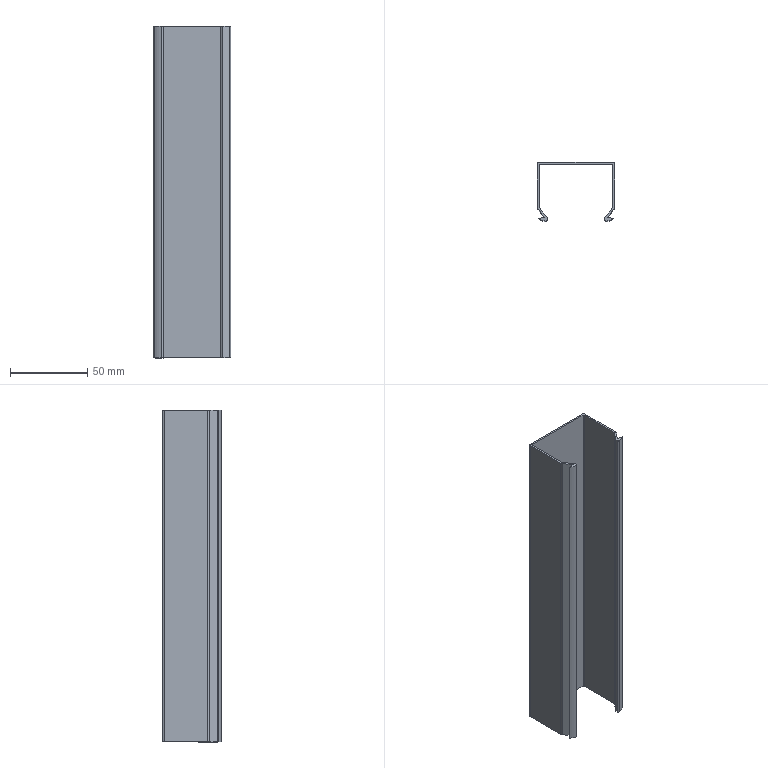Part | STEP file | 31E-01000CC12 | 1 solid | 28 faces | box 50 x 38.192 x 215 mm | volume 35398 mm3 | plane 16 | cylinder 12 | commonest cylinder face diameters 1 x4 2 x4 4 x2 26 x2
STEP:
#1=CARTESIAN_POINT('',(27.993,8.298,215.));
#2=VERTEX_POINT('',#1);
#3=CARTESIAN_POINT('',(32.281,3.187,215.));
#4=VERTEX_POINT('',#3);
#5=CARTESIAN_POINT('',(30.137,5.743,215.));
#6=DIRECTION('',(0.6428,-0.766,0.));
#7=VECTOR('',#6,1.);
#8=LINE('',#5,#7);
#9=EDGE_CURVE('',#2,#4,#8,.T.);
#10=ORIENTED_EDGE('',*,*,#9,.F.);
#11=CARTESIAN_POINT('',(27.993,8.298,0.));
#12=VERTEX_POINT('',#11);
#13=CARTESIAN_POINT('',(27.993,8.298,107.5));
#14=DIRECTION('',(0.,0.,-1.));
#15=VECTOR('',#14,1.);
#16=LINE('',#13,#15);
#17=EDGE_CURVE('',#2,#12,#16,.T.);
#18=ORIENTED_EDGE('',*,*,#17,.T.);
#19=CARTESIAN_POINT('',(32.281,3.187,0.));
#20=VERTEX_POINT('',#19);
#21=CARTESIAN_POINT('',(30.137,5.743,0.));
#22=DIRECTION('',(0.6428,-0.766,0.));
#23=VECTOR('',#22,1.);
#24=LINE('',#21,#23);
#25=EDGE_CURVE('',#12,#20,#24,.T.);
#26=ORIENTED_EDGE('',*,*,#25,.T.);
#27=CARTESIAN_POINT('',(32.281,3.187,107.5));
#28=DIRECTION('',(0.,0.,-1.));
#29=VECTOR('',#28,1.);
#30=LINE('',#27,#29);
#31=EDGE_CURVE('',#4,#20,#30,.T.);
#32=ORIENTED_EDGE('',*,*,#31,.F.);
#33=EDGE_LOOP('',(#10,#18,#26,#32));
#34=FACE_OUTER_BOUND('',#33,.T.);
#35=CARTESIAN_POINT('',(27.525,8.856,215.));
#36=DIRECTION('',(0.766,0.6428,0.));
#37=DIRECTION('',(-0.6428,0.766,0.));
#38=AXIS2_PLACEMENT_3D('',#35,#36,#37);
#39=PLANE('',#38);
#40=ADVANCED_FACE('',(#34),#39,.F.);
#41=CARTESIAN_POINT('',(76.325,9.293,215.));
#42=VERTEX_POINT('',#41);
#43=CARTESIAN_POINT('',(71.299,3.304,215.));
#44=VERTEX_POINT('',#43);
#45=CARTESIAN_POINT('',(73.812,6.298,215.));
#46=DIRECTION('',(-0.6428,-0.766,0.));
#47=VECTOR('',#46,1.);
#48=LINE('',#45,#47);
#49=EDGE_CURVE('',#42,#44,#48,.T.);
#50=ORIENTED_EDGE('',*,*,#49,.T.);
#51=CARTESIAN_POINT('',(71.182,2.983,215.));
#52=VERTEX_POINT('',#51);
#53=CARTESIAN_POINT('',(71.682,2.983,215.));
#54=DIRECTION('',(0.,0.,1.));
#55=AXIS2_PLACEMENT_3D('',#53,#54,$);
#56=CIRCLE('',#55,0.5);
#57=EDGE_CURVE('',#44,#52,#56,.T.);
#58=ORIENTED_EDGE('',*,*,#57,.T.);
#59=CARTESIAN_POINT('',(71.182,1.665,215.));
#60=VERTEX_POINT('',#59);
#61=CARTESIAN_POINT('',(71.182,2.324,215.));
#62=DIRECTION('',(0.,-1.,0.));
#63=VECTOR('',#62,1.);
#64=LINE('',#61,#63);
#65=EDGE_CURVE('',#52,#60,#64,.T.);
#66=ORIENTED_EDGE('',*,*,#65,.T.);
#67=CARTESIAN_POINT('',(72.397,0.6877,215.));
#68=VERTEX_POINT('',#67);
#69=CARTESIAN_POINT('',(72.182,1.665,215.));
#70=DIRECTION('',(0.,0.,1.));
#71=AXIS2_PLACEMENT_3D('',#69,#70,$);
#72=CIRCLE('',#71,1.);
#73=EDGE_CURVE('',#60,#68,#72,.T.);
#74=ORIENTED_EDGE('',*,*,#73,.T.);
#75=CARTESIAN_POINT('',(76.707,2.493,215.));
#76=VERTEX_POINT('',#75);
#77=CARTESIAN_POINT('',(69.613,13.386,215.));
#78=DIRECTION('',(0.,0.,1.));
#79=AXIS2_PLACEMENT_3D('',#77,#78,$);
#80=CIRCLE('',#79,13.);
#81=EDGE_CURVE('',#68,#76,#80,.T.);
#82=ORIENTED_EDGE('',*,*,#81,.T.);
#83=CARTESIAN_POINT('',(72.768,3.187,215.));
#84=VERTEX_POINT('',#83);
#85=CARTESIAN_POINT('',(74.738,2.84,215.));
#86=DIRECTION('',(-0.9848,0.1736,0.));
#87=VECTOR('',#86,1.);
#88=LINE('',#85,#87);
#89=EDGE_CURVE('',#76,#84,#88,.T.);
#90=ORIENTED_EDGE('',*,*,#89,.T.);
#91=CARTESIAN_POINT('',(77.057,8.298,215.));
#92=VERTEX_POINT('',#91);
#93=CARTESIAN_POINT('',(74.912,5.743,215.));
#94=DIRECTION('',(0.6428,0.766,0.));
#95=VECTOR('',#94,1.);
#96=LINE('',#93,#95);
#97=EDGE_CURVE('',#84,#92,#96,.T.);
#98=ORIENTED_EDGE('',*,*,#97,.T.);
#99=CARTESIAN_POINT('',(77.525,9.584,215.));
#100=VERTEX_POINT('',#99);
#101=CARTESIAN_POINT('',(75.525,9.584,215.));
#102=DIRECTION('',(0.,0.,1.));
#103=AXIS2_PLACEMENT_3D('',#101,#102,$);
#104=CIRCLE('',#103,2.);
#105=EDGE_CURVE('',#92,#100,#104,.T.);
#106=ORIENTED_EDGE('',*,*,#105,.T.);
#107=CARTESIAN_POINT('',(77.525,37.856,215.));
#108=VERTEX_POINT('',#107);
#109=CARTESIAN_POINT('',(77.525,23.72,215.));
#110=DIRECTION('',(0.,1.,0.));
#111=VECTOR('',#110,1.);
#112=LINE('',#109,#111);
#113=EDGE_CURVE('',#100,#108,#112,.T.);
#114=ORIENTED_EDGE('',*,*,#113,.T.);
#115=CARTESIAN_POINT('',(76.525,38.856,215.));
#116=VERTEX_POINT('',#115);
#117=CARTESIAN_POINT('',(76.525,37.856,215.));
#118=DIRECTION('',(0.,0.,1.));
#119=AXIS2_PLACEMENT_3D('',#117,#118,$);
#120=CIRCLE('',#119,1.);
#121=EDGE_CURVE('',#108,#116,#120,.T.);
#122=ORIENTED_EDGE('',*,*,#121,.T.);
#123=CARTESIAN_POINT('',(28.525,38.856,215.));
#124=VERTEX_POINT('',#123);
#125=CARTESIAN_POINT('',(52.525,38.856,215.));
#126=DIRECTION('',(-1.,0.,0.));
#127=VECTOR('',#126,1.);
#128=LINE('',#125,#127);
#129=EDGE_CURVE('',#116,#124,#128,.T.);
#130=ORIENTED_EDGE('',*,*,#129,.T.);
#131=CARTESIAN_POINT('',(27.525,37.856,215.));
#132=VERTEX_POINT('',#131);
#133=CARTESIAN_POINT('',(28.525,37.856,215.));
#134=DIRECTION('',(0.,0.,1.));
#135=AXIS2_PLACEMENT_3D('',#133,#134,$);
#136=CIRCLE('',#135,1.);
#137=EDGE_CURVE('',#124,#132,#136,.T.);
#138=ORIENTED_EDGE('',*,*,#137,.T.);
#139=CARTESIAN_POINT('',(27.525,9.584,215.));
#140=VERTEX_POINT('',#139);
#141=CARTESIAN_POINT('',(27.525,23.72,215.));
#142=DIRECTION('',(0.,-1.,0.));
#143=VECTOR('',#142,1.);
#144=LINE('',#141,#143);
#145=EDGE_CURVE('',#132,#140,#144,.T.);
#146=ORIENTED_EDGE('',*,*,#145,.T.);
#147=CARTESIAN_POINT('',(29.525,9.584,215.));
#148=DIRECTION('',(0.,0.,1.));
#149=AXIS2_PLACEMENT_3D('',#147,#148,$);
#150=CIRCLE('',#149,2.);
#151=EDGE_CURVE('',#140,#2,#150,.T.);
#152=ORIENTED_EDGE('',*,*,#151,.T.);
#153=ORIENTED_EDGE('',*,*,#9,.T.);
#154=CARTESIAN_POINT('',(28.342,2.493,215.));
#155=VERTEX_POINT('',#154);
#156=CARTESIAN_POINT('',(30.312,2.84,215.));
#157=DIRECTION('',(-0.9848,-0.1736,0.));
#158=VECTOR('',#157,1.);
#159=LINE('',#156,#158);
#160=EDGE_CURVE('',#4,#155,#159,.T.);
#161=ORIENTED_EDGE('',*,*,#160,.T.);
#162=CARTESIAN_POINT('',(32.653,0.6877,215.));
#163=VERTEX_POINT('',#162);
#164=CARTESIAN_POINT('',(35.437,13.386,215.));
#165=DIRECTION('',(0.,0.,1.));
#166=AXIS2_PLACEMENT_3D('',#164,#165,$);
#167=CIRCLE('',#166,13.);
#168=EDGE_CURVE('',#155,#163,#167,.T.);
#169=ORIENTED_EDGE('',*,*,#168,.T.);
#170=CARTESIAN_POINT('',(33.867,1.665,215.));
#171=VERTEX_POINT('',#170);
#172=CARTESIAN_POINT('',(32.867,1.665,215.));
#173=DIRECTION('',(0.,0.,1.));
#174=AXIS2_PLACEMENT_3D('',#172,#173,$);
#175=CIRCLE('',#174,1.);
#176=EDGE_CURVE('',#163,#171,#175,.T.);
#177=ORIENTED_EDGE('',*,*,#176,.T.);
#178=CARTESIAN_POINT('',(33.867,2.983,215.));
#179=VERTEX_POINT('',#178);
#180=CARTESIAN_POINT('',(33.867,2.324,215.));
#181=DIRECTION('',(0.,1.,0.));
#182=VECTOR('',#181,1.);
#183=LINE('',#180,#182);
#184=EDGE_CURVE('',#171,#179,#183,.T.);
#185=ORIENTED_EDGE('',*,*,#184,.T.);
#186=CARTESIAN_POINT('',(33.75,3.304,215.));
#187=VERTEX_POINT('',#186);
#188=CARTESIAN_POINT('',(33.367,2.983,215.));
#189=DIRECTION('',(0.,0.,1.));
#190=AXIS2_PLACEMENT_3D('',#188,#189,$);
#191=CIRCLE('',#190,0.5);
#192=EDGE_CURVE('',#179,#187,#191,.T.);
#193=ORIENTED_EDGE('',*,*,#192,.T.);
#194=CARTESIAN_POINT('',(28.725,9.293,215.));
#195=VERTEX_POINT('',#194);
#196=CARTESIAN_POINT('',(31.237,6.298,215.));
#197=DIRECTION('',(-0.6428,0.766,0.));
#198=VECTOR('',#197,1.);
#199=LINE('',#196,#198);
#200=EDGE_CURVE('',#187,#195,#199,.T.);
#201=ORIENTED_EDGE('',*,*,#200,.T.);
#202=CARTESIAN_POINT('',(28.725,37.156,215.));
#203=VERTEX_POINT('',#202);
#204=CARTESIAN_POINT('',(28.725,23.225,215.));
#205=DIRECTION('',(0.,1.,0.));
#206=VECTOR('',#205,1.);
#207=LINE('',#204,#206);
#208=EDGE_CURVE('',#195,#203,#207,.T.);
#209=ORIENTED_EDGE('',*,*,#208,.T.);
#210=CARTESIAN_POINT('',(29.225,37.656,215.));
#211=VERTEX_POINT('',#210);
#212=CARTESIAN_POINT('',(28.725,37.156,215.));
#213=CARTESIAN_POINT('',(28.725,37.219,215.));
#214=CARTESIAN_POINT('',(28.735,37.282,215.));
#215=CARTESIAN_POINT('',(28.754,37.343,215.));
#216=CARTESIAN_POINT('',(28.812,37.456,215.));
#217=CARTESIAN_POINT('',(28.902,37.546,215.));
#218=CARTESIAN_POINT('',(28.954,37.583,215.));
#219=CARTESIAN_POINT('',(29.039,37.627,215.));
#220=CARTESIAN_POINT('',(29.131,37.649,215.));
#221=CARTESIAN_POINT('',(29.162,37.654,215.));
#222=CARTESIAN_POINT('',(29.193,37.656,215.));
#223=CARTESIAN_POINT('',(29.225,37.656,215.));
#224=B_SPLINE_CURVE_WITH_KNOTS('',5,(#212,#213,#214,#215,#216,#217,#218,#219,#220,#221,#222,#223),.UNSPECIFIED.,.F.,.U.,(6,3,3,6),(0.,0.4443,0.8886,1.11),.UNSPECIFIED.);
#225=EDGE_CURVE('',#203,#211,#224,.T.);
#226=ORIENTED_EDGE('',*,*,#225,.T.);
#227=CARTESIAN_POINT('',(75.825,37.656,215.));
#228=VERTEX_POINT('',#227);
#229=CARTESIAN_POINT('',(52.525,37.656,215.));
#230=DIRECTION('',(1.,0.,0.));
#231=VECTOR('',#230,1.);
#232=LINE('',#229,#231);
#233=EDGE_CURVE('',#211,#228,#232,.T.);
#234=ORIENTED_EDGE('',*,*,#233,.T.);
#235=CARTESIAN_POINT('',(76.325,37.156,215.));
#236=VERTEX_POINT('',#235);
#237=CARTESIAN_POINT('',(75.825,37.656,215.));
#238=CARTESIAN_POINT('',(75.888,37.656,215.));
#239=CARTESIAN_POINT('',(75.95,37.646,215.));
#240=CARTESIAN_POINT('',(76.011,37.627,215.));
#241=CARTESIAN_POINT('',(76.124,37.569,215.));
#242=CARTESIAN_POINT('',(76.214,37.479,215.));
#243=CARTESIAN_POINT('',(76.252,37.427,215.));
#244=CARTESIAN_POINT('',(76.295,37.342,215.));
#245=CARTESIAN_POINT('',(76.317,37.25,215.));
#246=CARTESIAN_POINT('',(76.322,37.219,215.));
#247=CARTESIAN_POINT('',(76.325,37.187,215.));
#248=CARTESIAN_POINT('',(76.325,37.156,215.));
#249=B_SPLINE_CURVE_WITH_KNOTS('',5,(#237,#238,#239,#240,#241,#242,#243,#244,#245,#246,#247,#248),.UNSPECIFIED.,.F.,.U.,(6,3,3,6),(0.,0.4443,0.8886,1.11),.UNSPECIFIED.);
#250=EDGE_CURVE('',#228,#236,#249,.T.);
#251=ORIENTED_EDGE('',*,*,#250,.T.);
#252=CARTESIAN_POINT('',(76.325,23.225,215.));
#253=DIRECTION('',(0.,-1.,0.));
#254=VECTOR('',#253,1.);
#255=LINE('',#252,#254);
#256=EDGE_CURVE('',#236,#42,#255,.T.);
#257=ORIENTED_EDGE('',*,*,#256,.T.);
#258=EDGE_LOOP('',(#50,#58,#66,#74,#82,#90,#98,#106,#114,#122,#130,#138,#146,#152,#153,#161,#169,#177,#185,#193,#201,#209,#226,#234,#251,#257));
#259=FACE_OUTER_BOUND('',#258,.T.);
#260=CARTESIAN_POINT('',(35.437,13.386,215.));
#261=DIRECTION('',(0.,0.,1.));
#262=DIRECTION('',(1.,0.,0.));
#263=AXIS2_PLACEMENT_3D('',#260,#261,#262);
#264=PLANE('',#263);
#265=ADVANCED_FACE('',(#259),#264,.T.);
#266=ORIENTED_EDGE('',*,*,#151,.F.);
#267=CARTESIAN_POINT('',(27.525,9.584,0.));
#268=VERTEX_POINT('',#267);
#269=CARTESIAN_POINT('',(27.525,9.584,215.));
#270=DIRECTION('',(0.,0.,-1.));
#271=VECTOR('',#270,1.);
#272=LINE('',#269,#271);
#273=EDGE_CURVE('',#268,#140,#272,.F.);
#274=ORIENTED_EDGE('',*,*,#273,.F.);
#275=CARTESIAN_POINT('',(29.525,9.584,0.));
#276=DIRECTION('',(0.,0.,-1.));
#277=AXIS2_PLACEMENT_3D('',#275,#276,$);
#278=CIRCLE('',#277,2.);
#279=EDGE_CURVE('',#12,#268,#278,.T.);
#280=ORIENTED_EDGE('',*,*,#279,.F.);
#281=ORIENTED_EDGE('',*,*,#17,.F.);
#282=EDGE_LOOP('',(#266,#274,#280,#281));
#283=FACE_OUTER_BOUND('',#282,.T.);
#284=CARTESIAN_POINT('',(29.525,9.584,215.));
#285=DIRECTION('',(0.,0.,-1.));
#286=DIRECTION('',(1.,0.,0.));
#287=AXIS2_PLACEMENT_3D('',#284,#285,#286);
#288=CYLINDRICAL_SURFACE('',#287,2.);
#289=ADVANCED_FACE('',(#283),#288,.T.);
#290=CARTESIAN_POINT('',(71.182,2.983,0.));
#291=VERTEX_POINT('',#290);
#292=CARTESIAN_POINT('',(71.182,1.665,0.));
#293=VERTEX_POINT('',#292);
#294=CARTESIAN_POINT('',(71.182,2.324,0.));
#295=DIRECTION('',(0.,-1.,0.));
#296=VECTOR('',#295,1.);
#297=LINE('',#294,#296);
#298=EDGE_CURVE('',#291,#293,#297,.T.);
#299=ORIENTED_EDGE('',*,*,#298,.F.);
#300=CARTESIAN_POINT('',(71.299,3.304,0.));
#301=VERTEX_POINT('',#300);
#302=CARTESIAN_POINT('',(71.182,2.983,0.));
#303=CARTESIAN_POINT('',(71.182,3.038,0.));
#304=CARTESIAN_POINT('',(71.19,3.094,0.));
#305=CARTESIAN_POINT('',(71.206,3.149,0.));
#306=CARTESIAN_POINT('',(71.235,3.213,0.));
#307=CARTESIAN_POINT('',(71.274,3.271,0.));
#308=CARTESIAN_POINT('',(71.282,3.282,0.));
#309=CARTESIAN_POINT('',(71.29,3.293,0.));
#310=CARTESIAN_POINT('',(71.299,3.304,0.));
#311=B_SPLINE_CURVE_WITH_KNOTS('',5,(#302,#303,#304,#305,#306,#307,#308,#309,#310),.UNSPECIFIED.,.F.,.U.,(6,3,6),(0.,0.3949,0.4936),.UNSPECIFIED.);
#312=EDGE_CURVE('',#291,#301,#311,.T.);
#313=ORIENTED_EDGE('',*,*,#312,.T.);
#314=CARTESIAN_POINT('',(76.325,9.293,0.));
#315=VERTEX_POINT('',#314);
#316=CARTESIAN_POINT('',(73.812,6.298,0.));
#317=DIRECTION('',(-0.6428,-0.766,0.));
#318=VECTOR('',#317,1.);
#319=LINE('',#316,#318);
#320=EDGE_CURVE('',#315,#301,#319,.T.);
#321=ORIENTED_EDGE('',*,*,#320,.F.);
#322=CARTESIAN_POINT('',(76.325,37.156,0.));
#323=VERTEX_POINT('',#322);
#324=CARTESIAN_POINT('',(76.325,23.225,0.));
#325=DIRECTION('',(0.,-1.,0.));
#326=VECTOR('',#325,1.);
#327=LINE('',#324,#326);
#328=EDGE_CURVE('',#323,#315,#327,.T.);
#329=ORIENTED_EDGE('',*,*,#328,.F.);
#330=CARTESIAN_POINT('',(75.825,37.656,0.));
#331=VERTEX_POINT('',#330);
#332=CARTESIAN_POINT('',(75.825,37.156,0.));
#333=DIRECTION('',(0.,0.,1.));
#334=AXIS2_PLACEMENT_3D('',#332,#333,$);
#335=CIRCLE('',#334,0.5);
#336=EDGE_CURVE('',#323,#331,#335,.T.);
#337=ORIENTED_EDGE('',*,*,#336,.T.);
#338=CARTESIAN_POINT('',(29.225,37.656,0.));
#339=VERTEX_POINT('',#338);
#340=CARTESIAN_POINT('',(52.525,37.656,0.));
#341=DIRECTION('',(1.,0.,0.));
#342=VECTOR('',#341,1.);
#343=LINE('',#340,#342);
#344=EDGE_CURVE('',#339,#331,#343,.T.);
#345=ORIENTED_EDGE('',*,*,#344,.F.);
#346=CARTESIAN_POINT('',(28.725,37.156,0.));
#347=VERTEX_POINT('',#346);
#348=CARTESIAN_POINT('',(29.225,37.156,0.));
#349=DIRECTION('',(0.,0.,1.));
#350=AXIS2_PLACEMENT_3D('',#348,#349,$);
#351=CIRCLE('',#350,0.5);
#352=EDGE_CURVE('',#339,#347,#351,.T.);
#353=ORIENTED_EDGE('',*,*,#352,.T.);
#354=CARTESIAN_POINT('',(28.725,9.293,0.));
#355=VERTEX_POINT('',#354);
#356=CARTESIAN_POINT('',(28.725,23.225,0.));
#357=DIRECTION('',(0.,1.,0.));
#358=VECTOR('',#357,1.);
#359=LINE('',#356,#358);
#360=EDGE_CURVE('',#355,#347,#359,.T.);
#361=ORIENTED_EDGE('',*,*,#360,.F.);
#362=CARTESIAN_POINT('',(33.75,3.304,0.));
#363=VERTEX_POINT('',#362);
#364=CARTESIAN_POINT('',(31.237,6.298,0.));
#365=DIRECTION('',(-0.6428,0.766,0.));
#366=VECTOR('',#365,1.);
#367=LINE('',#364,#366);
#368=EDGE_CURVE('',#363,#355,#367,.T.);
#369=ORIENTED_EDGE('',*,*,#368,.F.);
#370=CARTESIAN_POINT('',(33.867,2.983,0.));
#371=VERTEX_POINT('',#370);
#372=CARTESIAN_POINT('',(33.75,3.304,0.));
#373=CARTESIAN_POINT('',(33.786,3.261,0.));
#374=CARTESIAN_POINT('',(33.816,3.213,0.));
#375=CARTESIAN_POINT('',(33.839,3.162,0.));
#376=CARTESIAN_POINT('',(33.858,3.094,0.));
#377=CARTESIAN_POINT('',(33.866,3.024,0.));
#378=CARTESIAN_POINT('',(33.867,3.01,0.));
#379=CARTESIAN_POINT('',(33.867,2.997,0.));
#380=CARTESIAN_POINT('',(33.867,2.983,0.));
#381=B_SPLINE_CURVE_WITH_KNOTS('',5,(#372,#373,#374,#375,#376,#377,#378,#379,#380),.UNSPECIFIED.,.F.,.U.,(6,3,6),(0.,0.3949,0.4936),.UNSPECIFIED.);
#382=EDGE_CURVE('',#363,#371,#381,.T.);
#383=ORIENTED_EDGE('',*,*,#382,.T.);
#384=CARTESIAN_POINT('',(33.867,1.665,0.));
#385=VERTEX_POINT('',#384);
#386=CARTESIAN_POINT('',(33.867,2.324,0.));
#387=DIRECTION('',(0.,1.,0.));
#388=VECTOR('',#387,1.);
#389=LINE('',#386,#388);
#390=EDGE_CURVE('',#385,#371,#389,.T.);
#391=ORIENTED_EDGE('',*,*,#390,.F.);
#392=CARTESIAN_POINT('',(32.653,0.6877,0.));
#393=VERTEX_POINT('',#392);
#394=CARTESIAN_POINT('',(32.867,1.665,0.));
#395=DIRECTION('',(0.,0.,1.));
#396=AXIS2_PLACEMENT_3D('',#394,#395,$);
#397=CIRCLE('',#396,1.);
#398=EDGE_CURVE('',#393,#385,#397,.T.);
#399=ORIENTED_EDGE('',*,*,#398,.F.);
#400=CARTESIAN_POINT('',(28.342,2.493,0.));
#401=VERTEX_POINT('',#400);
#402=CARTESIAN_POINT('',(35.437,13.386,0.));
#403=DIRECTION('',(0.,0.,1.));
#404=AXIS2_PLACEMENT_3D('',#402,#403,$);
#405=CIRCLE('',#404,13.);
#406=EDGE_CURVE('',#401,#393,#405,.T.);
#407=ORIENTED_EDGE('',*,*,#406,.F.);
#408=CARTESIAN_POINT('',(30.312,2.84,0.));
#409=DIRECTION('',(-0.9848,-0.1736,0.));
#410=VECTOR('',#409,1.);
#411=LINE('',#408,#410);
#412=EDGE_CURVE('',#20,#401,#411,.T.);
#413=ORIENTED_EDGE('',*,*,#412,.F.);
#414=ORIENTED_EDGE('',*,*,#25,.F.);
#415=ORIENTED_EDGE('',*,*,#279,.T.);
#416=CARTESIAN_POINT('',(27.525,37.856,0.));
#417=VERTEX_POINT('',#416);
#418=CARTESIAN_POINT('',(27.525,23.72,0.));
#419=DIRECTION('',(0.,-1.,0.));
#420=VECTOR('',#419,1.);
#421=LINE('',#418,#420);
#422=EDGE_CURVE('',#417,#268,#421,.T.);
#423=ORIENTED_EDGE('',*,*,#422,.F.);
#424=CARTESIAN_POINT('',(28.525,38.856,0.));
#425=VERTEX_POINT('',#424);
#426=CARTESIAN_POINT('',(27.525,37.856,0.));
#427=CARTESIAN_POINT('',(27.525,37.954,0.));
#428=CARTESIAN_POINT('',(27.537,38.052,0.));
#429=CARTESIAN_POINT('',(27.561,38.148,0.));
#430=CARTESIAN_POINT('',(27.632,38.332,0.));
#431=CARTESIAN_POINT('',(27.745,38.494,0.));
#432=CARTESIAN_POINT('',(27.812,38.567,0.));
#433=CARTESIAN_POINT('',(27.961,38.696,0.));
#434=CARTESIAN_POINT('',(28.137,38.786,0.));
#435=CARTESIAN_POINT('',(28.23,38.819,0.));
#436=CARTESIAN_POINT('',(28.346,38.846,0.));
#437=CARTESIAN_POINT('',(28.464,38.855,0.));
#438=CARTESIAN_POINT('',(28.484,38.856,0.));
#439=CARTESIAN_POINT('',(28.505,38.856,0.));
#440=CARTESIAN_POINT('',(28.525,38.856,0.));
#441=B_SPLINE_CURVE_WITH_KNOTS('',5,(#426,#427,#428,#429,#430,#431,#432,#433,#434,#435,#436,#437,#438,#439,#440),.UNSPECIFIED.,.F.,.U.,(6,3,3,3,6),(0.,0.6928,1.386,2.078,2.221),.UNSPECIFIED.);
#442=EDGE_CURVE('',#417,#425,#441,.T.);
#443=ORIENTED_EDGE('',*,*,#442,.T.);
#444=CARTESIAN_POINT('',(76.525,38.856,0.));
#445=VERTEX_POINT('',#444);
#446=CARTESIAN_POINT('',(52.525,38.856,0.));
#447=DIRECTION('',(-1.,0.,0.));
#448=VECTOR('',#447,1.);
#449=LINE('',#446,#448);
#450=EDGE_CURVE('',#445,#425,#449,.T.);
#451=ORIENTED_EDGE('',*,*,#450,.F.);
#452=CARTESIAN_POINT('',(77.525,37.856,0.));
#453=VERTEX_POINT('',#452);
#454=CARTESIAN_POINT('',(76.525,38.856,0.));
#455=CARTESIAN_POINT('',(76.623,38.856,0.));
#456=CARTESIAN_POINT('',(76.721,38.844,0.));
#457=CARTESIAN_POINT('',(76.817,38.82,0.));
#458=CARTESIAN_POINT('',(77.001,38.749,0.));
#459=CARTESIAN_POINT('',(77.163,38.636,0.));
#460=CARTESIAN_POINT('',(77.236,38.569,0.));
#461=CARTESIAN_POINT('',(77.365,38.42,0.));
#462=CARTESIAN_POINT('',(77.454,38.244,0.));
#463=CARTESIAN_POINT('',(77.488,38.151,0.));
#464=CARTESIAN_POINT('',(77.514,38.035,0.));
#465=CARTESIAN_POINT('',(77.523,37.917,0.));
#466=CARTESIAN_POINT('',(77.524,37.897,0.));
#467=CARTESIAN_POINT('',(77.525,37.876,0.));
#468=CARTESIAN_POINT('',(77.525,37.856,0.));
#469=B_SPLINE_CURVE_WITH_KNOTS('',5,(#454,#455,#456,#457,#458,#459,#460,#461,#462,#463,#464,#465,#466,#467,#468),.UNSPECIFIED.,.F.,.U.,(6,3,3,3,6),(0.,0.6928,1.386,2.078,2.221),.UNSPECIFIED.);
#470=EDGE_CURVE('',#445,#453,#469,.T.);
#471=ORIENTED_EDGE('',*,*,#470,.T.);
#472=CARTESIAN_POINT('',(77.525,9.584,0.));
#473=VERTEX_POINT('',#472);
#474=CARTESIAN_POINT('',(77.525,23.72,0.));
#475=DIRECTION('',(0.,1.,0.));
#476=VECTOR('',#475,1.);
#477=LINE('',#474,#476);
#478=EDGE_CURVE('',#473,#453,#477,.T.);
#479=ORIENTED_EDGE('',*,*,#478,.F.);
#480=CARTESIAN_POINT('',(77.057,8.298,0.));
#481=VERTEX_POINT('',#480);
#482=CARTESIAN_POINT('',(77.525,9.584,0.));
#483=CARTESIAN_POINT('',(77.525,9.361,0.));
#484=CARTESIAN_POINT('',(77.494,9.137,0.));
#485=CARTESIAN_POINT('',(77.431,8.92,0.));
#486=CARTESIAN_POINT('',(77.316,8.662,0.));
#487=CARTESIAN_POINT('',(77.16,8.431,0.));
#488=CARTESIAN_POINT('',(77.127,8.385,0.));
#489=CARTESIAN_POINT('',(77.093,8.341,0.));
#490=CARTESIAN_POINT('',(77.057,8.298,0.));
#491=B_SPLINE_CURVE_WITH_KNOTS('',5,(#482,#483,#484,#485,#486,#487,#488,#489,#490),.UNSPECIFIED.,.F.,.U.,(6,3,6),(0.,1.58,1.974),.UNSPECIFIED.);
#492=EDGE_CURVE('',#473,#481,#491,.T.);
#493=ORIENTED_EDGE('',*,*,#492,.T.);
#494=CARTESIAN_POINT('',(72.768,3.187,0.));
#495=VERTEX_POINT('',#494);
#496=CARTESIAN_POINT('',(74.912,5.743,0.));
#497=DIRECTION('',(0.6428,0.766,0.));
#498=VECTOR('',#497,1.);
#499=LINE('',#496,#498);
#500=EDGE_CURVE('',#495,#481,#499,.T.);
#501=ORIENTED_EDGE('',*,*,#500,.F.);
#502=CARTESIAN_POINT('',(76.707,2.493,0.));
#503=VERTEX_POINT('',#502);
#504=CARTESIAN_POINT('',(74.738,2.84,0.));
#505=DIRECTION('',(-0.9848,0.1736,0.));
#506=VECTOR('',#505,1.);
#507=LINE('',#504,#506);
#508=EDGE_CURVE('',#503,#495,#507,.T.);
#509=ORIENTED_EDGE('',*,*,#508,.F.);
#510=CARTESIAN_POINT('',(72.397,0.6877,0.));
#511=VERTEX_POINT('',#510);
#512=CARTESIAN_POINT('',(69.613,13.386,0.));
#513=DIRECTION('',(0.,0.,1.));
#514=AXIS2_PLACEMENT_3D('',#512,#513,$);
#515=CIRCLE('',#514,13.);
#516=EDGE_CURVE('',#511,#503,#515,.T.);
#517=ORIENTED_EDGE('',*,*,#516,.F.);
#518=CARTESIAN_POINT('',(72.182,1.665,0.));
#519=DIRECTION('',(0.,0.,1.));
#520=AXIS2_PLACEMENT_3D('',#518,#519,$);
#521=CIRCLE('',#520,1.);
#522=EDGE_CURVE('',#293,#511,#521,.T.);
#523=ORIENTED_EDGE('',*,*,#522,.F.);
#524=EDGE_LOOP('',(#299,#313,#321,#329,#337,#345,#353,#361,#369,#383,#391,#399,#407,#413,#414,#415,#423,#443,#451,#471,#479,#493,#501,#509,#517,#523));
#525=FACE_OUTER_BOUND('',#524,.T.);
#526=CARTESIAN_POINT('',(35.437,13.386,0.));
#527=DIRECTION('',(0.,0.,1.));
#528=DIRECTION('',(1.,0.,0.));
#529=AXIS2_PLACEMENT_3D('',#526,#527,#528);
#530=PLANE('',#529);
#531=ADVANCED_FACE('',(#525),#530,.F.);
#532=ORIENTED_EDGE('',*,*,#412,.T.);
#533=CARTESIAN_POINT('',(28.342,2.493,107.5));
#534=DIRECTION('',(0.,0.,-1.));
#535=VECTOR('',#534,1.);
#536=LINE('',#533,#535);
#537=EDGE_CURVE('',#155,#401,#536,.T.);
#538=ORIENTED_EDGE('',*,*,#537,.F.);
#539=ORIENTED_EDGE('',*,*,#160,.F.);
#540=ORIENTED_EDGE('',*,*,#31,.T.);
#541=EDGE_LOOP('',(#532,#538,#539,#540));
#542=FACE_OUTER_BOUND('',#541,.T.);
#543=CARTESIAN_POINT('',(32.281,3.187,215.));
#544=DIRECTION('',(0.1736,-0.9848,0.));
#545=DIRECTION('',(0.9848,0.1736,0.));
#546=AXIS2_PLACEMENT_3D('',#543,#544,#545);
#547=PLANE('',#546);
#548=ADVANCED_FACE('',(#542),#547,.F.);
#549=ORIENTED_EDGE('',*,*,#320,.T.);
#550=CARTESIAN_POINT('',(71.299,3.304,107.5));
#551=DIRECTION('',(0.,0.,1.));
#552=VECTOR('',#551,1.);
#553=LINE('',#550,#552);
#554=EDGE_CURVE('',#301,#44,#553,.T.);
#555=ORIENTED_EDGE('',*,*,#554,.T.);
#556=ORIENTED_EDGE('',*,*,#49,.F.);
#557=CARTESIAN_POINT('',(76.325,9.293,107.5));
#558=DIRECTION('',(0.,0.,-1.));
#559=VECTOR('',#558,1.);
#560=LINE('',#557,#559);
#561=EDGE_CURVE('',#42,#315,#560,.T.);
#562=ORIENTED_EDGE('',*,*,#561,.T.);
#563=EDGE_LOOP('',(#549,#555,#556,#562));
#564=FACE_OUTER_BOUND('',#563,.T.);
#565=CARTESIAN_POINT('',(76.325,9.293,215.));
#566=DIRECTION('',(0.766,-0.6428,0.));
#567=DIRECTION('',(0.6428,0.766,0.));
#568=AXIS2_PLACEMENT_3D('',#565,#566,#567);
#569=PLANE('',#568);
#570=ADVANCED_FACE('',(#564),#569,.F.);
#571=ORIENTED_EDGE('',*,*,#57,.F.);
#572=ORIENTED_EDGE('',*,*,#554,.F.);
#573=ORIENTED_EDGE('',*,*,#312,.F.);
#574=CARTESIAN_POINT('',(71.182,2.983,215.));
#575=DIRECTION('',(0.,0.,-1.));
#576=VECTOR('',#575,1.);
#577=LINE('',#574,#576);
#578=EDGE_CURVE('',#52,#291,#577,.T.);
#579=ORIENTED_EDGE('',*,*,#578,.F.);
#580=EDGE_LOOP('',(#571,#572,#573,#579));
#581=FACE_OUTER_BOUND('',#580,.T.);
#582=CARTESIAN_POINT('',(71.682,2.983,215.));
#583=DIRECTION('',(0.,0.,-1.));
#584=DIRECTION('',(-1.,0.,0.));
#585=AXIS2_PLACEMENT_3D('',#582,#583,#584);
#586=CYLINDRICAL_SURFACE('',#585,0.5);
#587=ADVANCED_FACE('',(#581),#586,.T.);
#588=ORIENTED_EDGE('',*,*,#65,.F.);
#589=ORIENTED_EDGE('',*,*,#578,.T.);
#590=ORIENTED_EDGE('',*,*,#298,.T.);
#591=CARTESIAN_POINT('',(71.182,1.665,107.5));
#592=DIRECTION('',(0.,0.,-1.));
#593=VECTOR('',#592,1.);
#594=LINE('',#591,#593);
#595=EDGE_CURVE('',#60,#293,#594,.T.);
#596=ORIENTED_EDGE('',*,*,#595,.F.);
#597=EDGE_LOOP('',(#588,#589,#590,#596));
#598=FACE_OUTER_BOUND('',#597,.T.);
#599=CARTESIAN_POINT('',(71.182,1.665,215.));
#600=DIRECTION('',(1.,0.,0.));
#601=DIRECTION('',(0.,0.,-1.));
#602=AXIS2_PLACEMENT_3D('',#599,#600,#601);
#603=PLANE('',#602);
#604=ADVANCED_FACE('',(#598),#603,.F.);
#605=ORIENTED_EDGE('',*,*,#522,.T.);
#606=CARTESIAN_POINT('',(72.397,0.6877,215.));
#607=DIRECTION('',(0.,0.,-1.));
#608=VECTOR('',#607,1.);
#609=LINE('',#606,#608);
#610=EDGE_CURVE('',#68,#511,#609,.T.);
#611=ORIENTED_EDGE('',*,*,#610,.F.);
#612=ORIENTED_EDGE('',*,*,#73,.F.);
#613=ORIENTED_EDGE('',*,*,#595,.T.);
#614=EDGE_LOOP('',(#605,#611,#612,#613));
#615=FACE_OUTER_BOUND('',#614,.T.);
#616=CARTESIAN_POINT('',(72.182,1.665,215.));
#617=DIRECTION('',(0.,0.,-1.));
#618=DIRECTION('',(1.,0.,0.));
#619=AXIS2_PLACEMENT_3D('',#616,#617,#618);
#620=CYLINDRICAL_SURFACE('',#619,1.);
#621=ADVANCED_FACE('',(#615),#620,.T.);
#622=ORIENTED_EDGE('',*,*,#516,.T.);
#623=CARTESIAN_POINT('',(76.707,2.493,215.));
#624=DIRECTION('',(0.,0.,-1.));
#625=VECTOR('',#624,1.);
#626=LINE('',#623,#625);
#627=EDGE_CURVE('',#76,#503,#626,.T.);
#628=ORIENTED_EDGE('',*,*,#627,.F.);
#629=ORIENTED_EDGE('',*,*,#81,.F.);
#630=ORIENTED_EDGE('',*,*,#610,.T.);
#631=EDGE_LOOP('',(#622,#628,#629,#630));
#632=FACE_OUTER_BOUND('',#631,.T.);
#633=CARTESIAN_POINT('',(69.613,13.386,215.));
#634=DIRECTION('',(0.,0.,-1.));
#635=DIRECTION('',(1.,0.,0.));
#636=AXIS2_PLACEMENT_3D('',#633,#634,#635);
#637=CYLINDRICAL_SURFACE('',#636,13.);
#638=ADVANCED_FACE('',(#632),#637,.T.);
#639=ORIENTED_EDGE('',*,*,#508,.T.);
#640=CARTESIAN_POINT('',(72.768,3.187,107.5));
#641=DIRECTION('',(0.,0.,-1.));
#642=VECTOR('',#641,1.);
#643=LINE('',#640,#642);
#644=EDGE_CURVE('',#84,#495,#643,.T.);
#645=ORIENTED_EDGE('',*,*,#644,.F.);
#646=ORIENTED_EDGE('',*,*,#89,.F.);
#647=ORIENTED_EDGE('',*,*,#627,.T.);
#648=EDGE_LOOP('',(#639,#645,#646,#647));
#649=FACE_OUTER_BOUND('',#648,.T.);
#650=CARTESIAN_POINT('',(72.768,3.187,215.));
#651=DIRECTION('',(-0.1736,-0.9848,0.));
#652=DIRECTION('',(0.9848,-0.1736,0.));
#653=AXIS2_PLACEMENT_3D('',#650,#651,#652);
#654=PLANE('',#653);
#655=ADVANCED_FACE('',(#649),#654,.F.);
#656=ORIENTED_EDGE('',*,*,#500,.T.);
#657=CARTESIAN_POINT('',(77.057,8.298,107.5));
#658=DIRECTION('',(0.,0.,1.));
#659=VECTOR('',#658,1.);
#660=LINE('',#657,#659);
#661=EDGE_CURVE('',#481,#92,#660,.T.);
#662=ORIENTED_EDGE('',*,*,#661,.T.);
#663=ORIENTED_EDGE('',*,*,#97,.F.);
#664=ORIENTED_EDGE('',*,*,#644,.T.);
#665=EDGE_LOOP('',(#656,#662,#663,#664));
#666=FACE_OUTER_BOUND('',#665,.T.);
#667=CARTESIAN_POINT('',(77.525,8.856,215.));
#668=DIRECTION('',(-0.766,0.6428,0.));
#669=DIRECTION('',(-0.6428,-0.766,0.));
#670=AXIS2_PLACEMENT_3D('',#667,#668,#669);
#671=PLANE('',#670);
#672=ADVANCED_FACE('',(#666),#671,.F.);
#673=ORIENTED_EDGE('',*,*,#105,.F.);
#674=ORIENTED_EDGE('',*,*,#661,.F.);
#675=ORIENTED_EDGE('',*,*,#492,.F.);
#676=CARTESIAN_POINT('',(77.525,9.584,215.));
#677=DIRECTION('',(0.,0.,-1.));
#678=VECTOR('',#677,1.);
#679=LINE('',#676,#678);
#680=EDGE_CURVE('',#100,#473,#679,.T.);
#681=ORIENTED_EDGE('',*,*,#680,.F.);
#682=EDGE_LOOP('',(#673,#674,#675,#681));
#683=FACE_OUTER_BOUND('',#682,.T.);
#684=CARTESIAN_POINT('',(75.525,9.584,215.));
#685=DIRECTION('',(0.,0.,-1.));
#686=DIRECTION('',(1.,0.,0.));
#687=AXIS2_PLACEMENT_3D('',#684,#685,#686);
#688=CYLINDRICAL_SURFACE('',#687,2.);
#689=ADVANCED_FACE('',(#683),#688,.T.);
#690=ORIENTED_EDGE('',*,*,#478,.T.);
#691=CARTESIAN_POINT('',(77.525,37.856,107.5));
#692=DIRECTION('',(0.,0.,1.));
#693=VECTOR('',#692,1.);
#694=LINE('',#691,#693);
#695=EDGE_CURVE('',#453,#108,#694,.T.);
#696=ORIENTED_EDGE('',*,*,#695,.T.);
#697=ORIENTED_EDGE('',*,*,#113,.F.);
#698=ORIENTED_EDGE('',*,*,#680,.T.);
#699=EDGE_LOOP('',(#690,#696,#697,#698));
#700=FACE_OUTER_BOUND('',#699,.T.);
#701=CARTESIAN_POINT('',(77.525,8.856,215.));
#702=DIRECTION('',(-1.,0.,0.));
#703=DIRECTION('',(0.,0.,1.));
#704=AXIS2_PLACEMENT_3D('',#701,#702,#703);
#705=PLANE('',#704);
#706=ADVANCED_FACE('',(#700),#705,.F.);
#707=ORIENTED_EDGE('',*,*,#121,.F.);
#708=ORIENTED_EDGE('',*,*,#695,.F.);
#709=ORIENTED_EDGE('',*,*,#470,.F.);
#710=CARTESIAN_POINT('',(76.525,38.856,215.));
#711=DIRECTION('',(0.,0.,-1.));
#712=VECTOR('',#711,1.);
#713=LINE('',#710,#712);
#714=EDGE_CURVE('',#116,#445,#713,.T.);
#715=ORIENTED_EDGE('',*,*,#714,.F.);
#716=EDGE_LOOP('',(#707,#708,#709,#715));
#717=FACE_OUTER_BOUND('',#716,.T.);
#718=CARTESIAN_POINT('',(76.525,37.856,215.));
#719=DIRECTION('',(0.,0.,-1.));
#720=DIRECTION('',(-1.,0.,0.));
#721=AXIS2_PLACEMENT_3D('',#718,#719,#720);
#722=CYLINDRICAL_SURFACE('',#721,1.);
#723=ADVANCED_FACE('',(#717),#722,.T.);
#724=ORIENTED_EDGE('',*,*,#129,.F.);
#725=ORIENTED_EDGE('',*,*,#714,.T.);
#726=ORIENTED_EDGE('',*,*,#450,.T.);
#727=CARTESIAN_POINT('',(28.525,38.856,107.5));
#728=DIRECTION('',(0.,0.,1.));
#729=VECTOR('',#728,1.);
#730=LINE('',#727,#729);
#731=EDGE_CURVE('',#425,#124,#730,.T.);
#732=ORIENTED_EDGE('',*,*,#731,.T.);
#733=EDGE_LOOP('',(#724,#725,#726,#732));
#734=FACE_OUTER_BOUND('',#733,.T.);
#735=CARTESIAN_POINT('',(27.525,38.856,215.));
#736=DIRECTION('',(0.,-1.,0.));
#737=DIRECTION('',(1.,0.,0.));
#738=AXIS2_PLACEMENT_3D('',#735,#736,#737);
#739=PLANE('',#738);
#740=ADVANCED_FACE('',(#734),#739,.F.);
#741=ORIENTED_EDGE('',*,*,#137,.F.);
#742=ORIENTED_EDGE('',*,*,#731,.F.);
#743=ORIENTED_EDGE('',*,*,#442,.F.);
#744=CARTESIAN_POINT('',(27.525,37.856,215.));
#745=DIRECTION('',(0.,0.,-1.));
#746=VECTOR('',#745,1.);
#747=LINE('',#744,#746);
#748=EDGE_CURVE('',#132,#417,#747,.T.);
#749=ORIENTED_EDGE('',*,*,#748,.F.);
#750=EDGE_LOOP('',(#741,#742,#743,#749));
#751=FACE_OUTER_BOUND('',#750,.T.);
#752=CARTESIAN_POINT('',(28.525,37.856,215.));
#753=DIRECTION('',(0.,0.,-1.));
#754=DIRECTION('',(-1.,0.,0.));
#755=AXIS2_PLACEMENT_3D('',#752,#753,#754);
#756=CYLINDRICAL_SURFACE('',#755,1.);
#757=ADVANCED_FACE('',(#751),#756,.T.);
#758=ORIENTED_EDGE('',*,*,#145,.F.);
#759=ORIENTED_EDGE('',*,*,#748,.T.);
#760=ORIENTED_EDGE('',*,*,#422,.T.);
#761=ORIENTED_EDGE('',*,*,#273,.T.);
#762=EDGE_LOOP('',(#758,#759,#760,#761));
#763=FACE_OUTER_BOUND('',#762,.T.);
#764=CARTESIAN_POINT('',(27.525,8.856,215.));
#765=DIRECTION('',(1.,0.,0.));
#766=DIRECTION('',(0.,0.,-1.));
#767=AXIS2_PLACEMENT_3D('',#764,#765,#766);
#768=PLANE('',#767);
#769=ADVANCED_FACE('',(#763),#768,.F.);
#770=ORIENTED_EDGE('',*,*,#406,.T.);
#771=CARTESIAN_POINT('',(32.653,0.6877,215.));
#772=DIRECTION('',(0.,0.,-1.));
#773=VECTOR('',#772,1.);
#774=LINE('',#771,#773);
#775=EDGE_CURVE('',#163,#393,#774,.T.);
#776=ORIENTED_EDGE('',*,*,#775,.F.);
#777=ORIENTED_EDGE('',*,*,#168,.F.);
#778=ORIENTED_EDGE('',*,*,#537,.T.);
#779=EDGE_LOOP('',(#770,#776,#777,#778));
#780=FACE_OUTER_BOUND('',#779,.T.);
#781=CARTESIAN_POINT('',(35.437,13.386,215.));
#782=DIRECTION('',(0.,0.,-1.));
#783=DIRECTION('',(1.,0.,0.));
#784=AXIS2_PLACEMENT_3D('',#781,#782,#783);
#785=CYLINDRICAL_SURFACE('',#784,13.);
#786=ADVANCED_FACE('',(#780),#785,.T.);
#787=ORIENTED_EDGE('',*,*,#398,.T.);
#788=CARTESIAN_POINT('',(33.867,1.665,215.));
#789=DIRECTION('',(0.,0.,-1.));
#790=VECTOR('',#789,1.);
#791=LINE('',#788,#790);
#792=EDGE_CURVE('',#171,#385,#791,.T.);
#793=ORIENTED_EDGE('',*,*,#792,.F.);
#794=ORIENTED_EDGE('',*,*,#176,.F.);
#795=ORIENTED_EDGE('',*,*,#775,.T.);
#796=EDGE_LOOP('',(#787,#793,#794,#795));
#797=FACE_OUTER_BOUND('',#796,.T.);
#798=CARTESIAN_POINT('',(32.867,1.665,215.));
#799=DIRECTION('',(0.,0.,-1.));
#800=DIRECTION('',(1.,0.,0.));
#801=AXIS2_PLACEMENT_3D('',#798,#799,#800);
#802=CYLINDRICAL_SURFACE('',#801,1.);
#803=ADVANCED_FACE('',(#797),#802,.T.);
#804=ORIENTED_EDGE('',*,*,#390,.T.);
#805=CARTESIAN_POINT('',(33.867,2.983,107.5));
#806=DIRECTION('',(0.,0.,1.));
#807=VECTOR('',#806,1.);
#808=LINE('',#805,#807);
#809=EDGE_CURVE('',#371,#179,#808,.T.);
#810=ORIENTED_EDGE('',*,*,#809,.T.);
#811=ORIENTED_EDGE('',*,*,#184,.F.);
#812=ORIENTED_EDGE('',*,*,#792,.T.);
#813=EDGE_LOOP('',(#804,#810,#811,#812));
#814=FACE_OUTER_BOUND('',#813,.T.);
#815=CARTESIAN_POINT('',(33.867,1.665,215.));
#816=DIRECTION('',(-1.,0.,0.));
#817=DIRECTION('',(0.,0.,1.));
#818=AXIS2_PLACEMENT_3D('',#815,#816,#817);
#819=PLANE('',#818);
#820=ADVANCED_FACE('',(#814),#819,.F.);
#821=ORIENTED_EDGE('',*,*,#192,.F.);
#822=ORIENTED_EDGE('',*,*,#809,.F.);
#823=ORIENTED_EDGE('',*,*,#382,.F.);
#824=CARTESIAN_POINT('',(33.75,3.304,215.));
#825=DIRECTION('',(0.,0.,-1.));
#826=VECTOR('',#825,1.);
#827=LINE('',#824,#826);
#828=EDGE_CURVE('',#187,#363,#827,.T.);
#829=ORIENTED_EDGE('',*,*,#828,.F.);
#830=EDGE_LOOP('',(#821,#822,#823,#829));
#831=FACE_OUTER_BOUND('',#830,.T.);
#832=CARTESIAN_POINT('',(33.367,2.983,215.));
#833=DIRECTION('',(0.,0.,-1.));
#834=DIRECTION('',(-1.,0.,0.));
#835=AXIS2_PLACEMENT_3D('',#832,#833,#834);
#836=CYLINDRICAL_SURFACE('',#835,0.5);
#837=ADVANCED_FACE('',(#831),#836,.T.);
#838=ORIENTED_EDGE('',*,*,#200,.F.);
#839=ORIENTED_EDGE('',*,*,#828,.T.);
#840=ORIENTED_EDGE('',*,*,#368,.T.);
#841=CARTESIAN_POINT('',(28.725,9.293,107.5));
#842=DIRECTION('',(0.,0.,-1.));
#843=VECTOR('',#842,1.);
#844=LINE('',#841,#843);
#845=EDGE_CURVE('',#195,#355,#844,.T.);
#846=ORIENTED_EDGE('',*,*,#845,.F.);
#847=EDGE_LOOP('',(#838,#839,#840,#846));
#848=FACE_OUTER_BOUND('',#847,.T.);
#849=CARTESIAN_POINT('',(28.725,9.293,215.));
#850=DIRECTION('',(-0.766,-0.6428,0.));
#851=DIRECTION('',(0.6428,-0.766,0.));
#852=AXIS2_PLACEMENT_3D('',#849,#850,#851);
#853=PLANE('',#852);
#854=ADVANCED_FACE('',(#848),#853,.F.);
#855=ORIENTED_EDGE('',*,*,#360,.T.);
#856=CARTESIAN_POINT('',(28.725,37.156,107.5));
#857=DIRECTION('',(0.,0.,1.));
#858=VECTOR('',#857,1.);
#859=LINE('',#856,#858);
#860=EDGE_CURVE('',#347,#203,#859,.T.);
#861=ORIENTED_EDGE('',*,*,#860,.T.);
#862=ORIENTED_EDGE('',*,*,#208,.F.);
#863=ORIENTED_EDGE('',*,*,#845,.T.);
#864=EDGE_LOOP('',(#855,#861,#862,#863));
#865=FACE_OUTER_BOUND('',#864,.T.);
#866=CARTESIAN_POINT('',(28.725,9.293,215.));
#867=DIRECTION('',(-1.,0.,0.));
#868=DIRECTION('',(0.,0.,1.));
#869=AXIS2_PLACEMENT_3D('',#866,#867,#868);
#870=PLANE('',#869);
#871=ADVANCED_FACE('',(#865),#870,.F.);
#872=ORIENTED_EDGE('',*,*,#225,.F.);
#873=ORIENTED_EDGE('',*,*,#860,.F.);
#874=ORIENTED_EDGE('',*,*,#352,.F.);
#875=CARTESIAN_POINT('',(29.225,37.656,215.));
#876=DIRECTION('',(0.,0.,1.));
#877=VECTOR('',#876,1.);
#878=LINE('',#875,#877);
#879=EDGE_CURVE('',#211,#339,#878,.F.);
#880=ORIENTED_EDGE('',*,*,#879,.F.);
#881=EDGE_LOOP('',(#872,#873,#874,#880));
#882=FACE_OUTER_BOUND('',#881,.T.);
#883=CARTESIAN_POINT('',(29.225,37.156,215.));
#884=DIRECTION('',(0.,0.,1.));
#885=DIRECTION('',(1.,0.,0.));
#886=AXIS2_PLACEMENT_3D('',#883,#884,#885);
#887=CYLINDRICAL_SURFACE('',#886,0.5);
#888=ADVANCED_FACE('',(#882),#887,.F.);
#889=ORIENTED_EDGE('',*,*,#344,.T.);
#890=CARTESIAN_POINT('',(75.825,37.656,107.5));
#891=DIRECTION('',(0.,0.,1.));
#892=VECTOR('',#891,1.);
#893=LINE('',#890,#892);
#894=EDGE_CURVE('',#331,#228,#893,.T.);
#895=ORIENTED_EDGE('',*,*,#894,.T.);
#896=ORIENTED_EDGE('',*,*,#233,.F.);
#897=ORIENTED_EDGE('',*,*,#879,.T.);
#898=EDGE_LOOP('',(#889,#895,#896,#897));
#899=FACE_OUTER_BOUND('',#898,.T.);
#900=CARTESIAN_POINT('',(28.725,37.656,215.));
#901=DIRECTION('',(0.,1.,0.));
#902=DIRECTION('',(-1.,0.,0.));
#903=AXIS2_PLACEMENT_3D('',#900,#901,#902);
#904=PLANE('',#903);
#905=ADVANCED_FACE('',(#899),#904,.F.);
#906=ORIENTED_EDGE('',*,*,#250,.F.);
#907=ORIENTED_EDGE('',*,*,#894,.F.);
#908=ORIENTED_EDGE('',*,*,#336,.F.);
#909=CARTESIAN_POINT('',(76.325,37.156,215.));
#910=DIRECTION('',(0.,0.,1.));
#911=VECTOR('',#910,1.);
#912=LINE('',#909,#911);
#913=EDGE_CURVE('',#236,#323,#912,.F.);
#914=ORIENTED_EDGE('',*,*,#913,.F.);
#915=EDGE_LOOP('',(#906,#907,#908,#914));
#916=FACE_OUTER_BOUND('',#915,.T.);
#917=CARTESIAN_POINT('',(75.825,37.156,215.));
#918=DIRECTION('',(0.,0.,1.));
#919=DIRECTION('',(1.,0.,0.));
#920=AXIS2_PLACEMENT_3D('',#917,#918,#919);
#921=CYLINDRICAL_SURFACE('',#920,0.5);
#922=ADVANCED_FACE('',(#916),#921,.F.);
#923=ORIENTED_EDGE('',*,*,#256,.F.);
#924=ORIENTED_EDGE('',*,*,#913,.T.);
#925=ORIENTED_EDGE('',*,*,#328,.T.);
#926=ORIENTED_EDGE('',*,*,#561,.F.);
#927=EDGE_LOOP('',(#923,#924,#925,#926));
#928=FACE_OUTER_BOUND('',#927,.T.);
#929=CARTESIAN_POINT('',(76.325,9.293,215.));
#930=DIRECTION('',(1.,0.,0.));
#931=DIRECTION('',(0.,1.,0.));
#932=AXIS2_PLACEMENT_3D('',#929,#930,#931);
#933=PLANE('',#932);
#934=ADVANCED_FACE('',(#928),#933,.F.);
#935=CLOSED_SHELL('',(#40,#265,#289,#531,#548,#570,#587,#604,#621,#638,#655,#672,#689,#706,#723,#740,#757,#769,#786,#803,#820,#837,#854,#871,#888,#905,#922,#934));
#936=MANIFOLD_SOLID_BREP('',#935);
#937=(LENGTH_UNIT()NAMED_UNIT(*)SI_UNIT(.MILLI.,.METRE.));
#938=UNCERTAINTY_MEASURE_WITH_UNIT(LENGTH_MEASURE(0.005),#937,'','');
#939=(NAMED_UNIT(*)PLANE_ANGLE_UNIT()SI_UNIT($,.RADIAN.));
#940=(NAMED_UNIT(*)SI_UNIT($,.STERADIAN.)SOLID_ANGLE_UNIT());
#941=(GEOMETRIC_REPRESENTATION_CONTEXT(3)GLOBAL_UNCERTAINTY_ASSIGNED_CONTEXT((#938))GLOBAL_UNIT_ASSIGNED_CONTEXT((#937,#939,#940))REPRESENTATION_CONTEXT('',''));
#942=ADVANCED_BREP_SHAPE_REPRESENTATION('',(#936),#941);